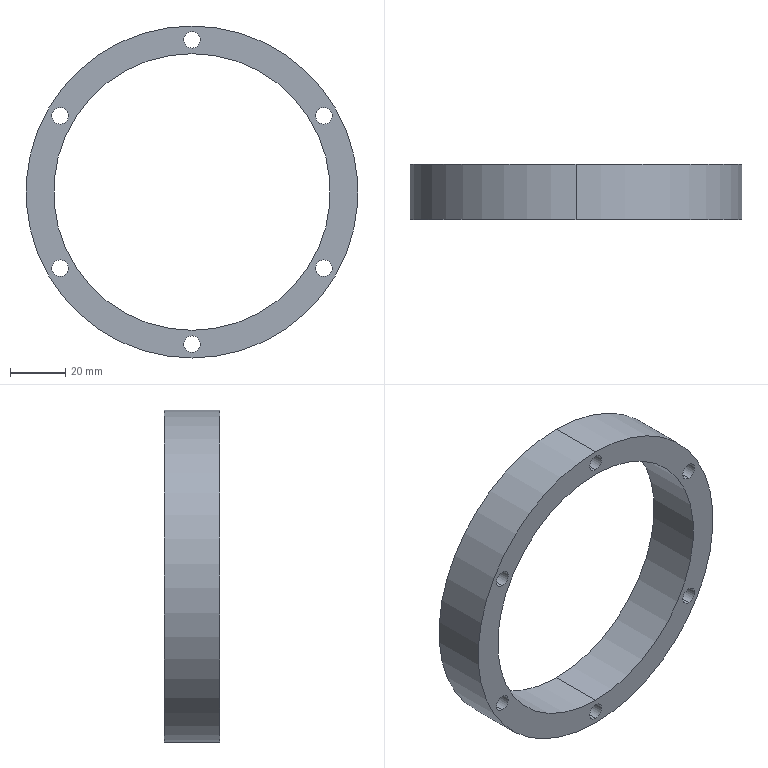Part | SolidWorks | features CirPattern 1, Extrusion 1, ICE 1 | 1 solid | 18 faces | box 120 x 20 x 120 mm | volume 65722 mm3 | cylinder 16 | plane 2 | commonest cylinder face diameters 6 x12 100 x2 120 x2
STEP:
#1=CARTESIAN_POINT('',(-47.631,0.,-30.5));
#2=VERTEX_POINT('',#1);
#3=CARTESIAN_POINT('',(-47.631,0.,-24.5));
#4=VERTEX_POINT('',#3);
#5=CARTESIAN_POINT('',(-47.631,0.,-27.5));
#6=DIRECTION('',(0.,1.,0.));
#7=DIRECTION('',(0.866,0.,0.5));
#8=AXIS2_PLACEMENT_3D('',#5,#6,#7);
#9=CIRCLE('',#8,3.);
#10=EDGE_CURVE('',#2,#4,#9,.T.);
#11=ORIENTED_EDGE('',*,*,#10,.F.);
#12=CARTESIAN_POINT('',(-47.631,20.,-30.5));
#13=VERTEX_POINT('',#12);
#14=CARTESIAN_POINT('',(-47.631,0.,-30.5));
#15=DIRECTION('',(0.,1.,0.));
#16=VECTOR('',#15,1000.);
#17=LINE('',#14,#16);
#18=EDGE_CURVE('',#2,#13,#17,.T.);
#19=ORIENTED_EDGE('',*,*,#18,.T.);
#20=CARTESIAN_POINT('',(-47.631,20.,-24.5));
#21=VERTEX_POINT('',#20);
#22=CARTESIAN_POINT('',(-47.631,20.,-27.5));
#23=DIRECTION('',(0.,1.,0.));
#24=DIRECTION('',(0.866,0.,0.5));
#25=AXIS2_PLACEMENT_3D('',#22,#23,#24);
#26=CIRCLE('',#25,3.);
#27=EDGE_CURVE('',#13,#21,#26,.T.);
#28=ORIENTED_EDGE('',*,*,#27,.T.);
#29=CARTESIAN_POINT('',(-47.631,0.,-24.5));
#30=DIRECTION('',(0.,1.,0.));
#31=VECTOR('',#30,1000.);
#32=LINE('',#29,#31);
#33=EDGE_CURVE('',#4,#21,#32,.T.);
#34=ORIENTED_EDGE('',*,*,#33,.F.);
#35=EDGE_LOOP('',(#11,#19,#28,#34));
#36=FACE_OUTER_BOUND('',#35,.T.);
#37=CARTESIAN_POINT('',(-47.631,0.,-27.5));
#38=DIRECTION('',(0.,1.,0.));
#39=DIRECTION('',(0.,0.,1.));
#40=AXIS2_PLACEMENT_3D('',#37,#38,#39);
#41=CYLINDRICAL_SURFACE('',#40,3.);
#42=ADVANCED_FACE('',(#36),#41,.F.);
#43=CARTESIAN_POINT('',(-47.631,0.,24.5));
#44=VERTEX_POINT('',#43);
#45=CARTESIAN_POINT('',(-47.631,0.,30.5));
#46=VERTEX_POINT('',#45);
#47=CARTESIAN_POINT('',(-47.631,0.,27.5));
#48=DIRECTION('',(0.,1.,0.));
#49=DIRECTION('',(0.866,0.,-0.5));
#50=AXIS2_PLACEMENT_3D('',#47,#48,#49);
#51=CIRCLE('',#50,3.);
#52=EDGE_CURVE('',#44,#46,#51,.T.);
#53=ORIENTED_EDGE('',*,*,#52,.F.);
#54=CARTESIAN_POINT('',(-47.631,20.,24.5));
#55=VERTEX_POINT('',#54);
#56=CARTESIAN_POINT('',(-47.631,0.,24.5));
#57=DIRECTION('',(0.,1.,0.));
#58=VECTOR('',#57,1000.);
#59=LINE('',#56,#58);
#60=EDGE_CURVE('',#44,#55,#59,.T.);
#61=ORIENTED_EDGE('',*,*,#60,.T.);
#62=CARTESIAN_POINT('',(-47.631,20.,30.5));
#63=VERTEX_POINT('',#62);
#64=CARTESIAN_POINT('',(-47.631,20.,27.5));
#65=DIRECTION('',(0.,1.,0.));
#66=DIRECTION('',(0.866,0.,-0.5));
#67=AXIS2_PLACEMENT_3D('',#64,#65,#66);
#68=CIRCLE('',#67,3.);
#69=EDGE_CURVE('',#55,#63,#68,.T.);
#70=ORIENTED_EDGE('',*,*,#69,.T.);
#71=CARTESIAN_POINT('',(-47.631,0.,30.5));
#72=DIRECTION('',(0.,1.,0.));
#73=VECTOR('',#72,1000.);
#74=LINE('',#71,#73);
#75=EDGE_CURVE('',#46,#63,#74,.T.);
#76=ORIENTED_EDGE('',*,*,#75,.F.);
#77=EDGE_LOOP('',(#53,#61,#70,#76));
#78=FACE_OUTER_BOUND('',#77,.T.);
#79=CARTESIAN_POINT('',(-47.631,0.,27.5));
#80=DIRECTION('',(0.,1.,0.));
#81=DIRECTION('',(0.,0.,1.));
#82=AXIS2_PLACEMENT_3D('',#79,#80,#81);
#83=CYLINDRICAL_SURFACE('',#82,3.);
#84=ADVANCED_FACE('',(#78),#83,.F.);
#85=CARTESIAN_POINT('',(0.,0.,52.));
#86=VERTEX_POINT('',#85);
#87=CARTESIAN_POINT('',(0.,0.,58.));
#88=VERTEX_POINT('',#87);
#89=CARTESIAN_POINT('',(0.,0.,55.));
#90=DIRECTION('',(0.,1.,0.));
#91=DIRECTION('',(0.,0.,-1.));
#92=AXIS2_PLACEMENT_3D('',#89,#90,#91);
#93=CIRCLE('',#92,3.);
#94=EDGE_CURVE('',#86,#88,#93,.T.);
#95=ORIENTED_EDGE('',*,*,#94,.F.);
#96=CARTESIAN_POINT('',(0.,20.,52.));
#97=VERTEX_POINT('',#96);
#98=CARTESIAN_POINT('',(0.,0.,52.));
#99=DIRECTION('',(0.,1.,0.));
#100=VECTOR('',#99,1000.);
#101=LINE('',#98,#100);
#102=EDGE_CURVE('',#86,#97,#101,.T.);
#103=ORIENTED_EDGE('',*,*,#102,.T.);
#104=CARTESIAN_POINT('',(0.,20.,58.));
#105=VERTEX_POINT('',#104);
#106=CARTESIAN_POINT('',(0.,20.,55.));
#107=DIRECTION('',(0.,1.,0.));
#108=DIRECTION('',(0.,0.,-1.));
#109=AXIS2_PLACEMENT_3D('',#106,#107,#108);
#110=CIRCLE('',#109,3.);
#111=EDGE_CURVE('',#97,#105,#110,.T.);
#112=ORIENTED_EDGE('',*,*,#111,.T.);
#113=CARTESIAN_POINT('',(0.,0.,58.));
#114=DIRECTION('',(0.,1.,0.));
#115=VECTOR('',#114,1000.);
#116=LINE('',#113,#115);
#117=EDGE_CURVE('',#88,#105,#116,.T.);
#118=ORIENTED_EDGE('',*,*,#117,.F.);
#119=EDGE_LOOP('',(#95,#103,#112,#118));
#120=FACE_OUTER_BOUND('',#119,.T.);
#121=CARTESIAN_POINT('',(0.,0.,55.));
#122=DIRECTION('',(0.,1.,0.));
#123=DIRECTION('',(0.,0.,1.));
#124=AXIS2_PLACEMENT_3D('',#121,#122,#123);
#125=CYLINDRICAL_SURFACE('',#124,3.);
#126=ADVANCED_FACE('',(#120),#125,.F.);
#127=CARTESIAN_POINT('',(47.631,0.,24.5));
#128=VERTEX_POINT('',#127);
#129=CARTESIAN_POINT('',(47.631,0.,30.5));
#130=VERTEX_POINT('',#129);
#131=CARTESIAN_POINT('',(47.631,0.,27.5));
#132=DIRECTION('',(0.,1.,0.));
#133=DIRECTION('',(-0.866,0.,-0.5));
#134=AXIS2_PLACEMENT_3D('',#131,#132,#133);
#135=CIRCLE('',#134,3.);
#136=EDGE_CURVE('',#128,#130,#135,.T.);
#137=ORIENTED_EDGE('',*,*,#136,.F.);
#138=CARTESIAN_POINT('',(47.631,20.,24.5));
#139=VERTEX_POINT('',#138);
#140=CARTESIAN_POINT('',(47.631,0.,24.5));
#141=DIRECTION('',(0.,1.,0.));
#142=VECTOR('',#141,1000.);
#143=LINE('',#140,#142);
#144=EDGE_CURVE('',#128,#139,#143,.T.);
#145=ORIENTED_EDGE('',*,*,#144,.T.);
#146=CARTESIAN_POINT('',(47.631,20.,30.5));
#147=VERTEX_POINT('',#146);
#148=CARTESIAN_POINT('',(47.631,20.,27.5));
#149=DIRECTION('',(0.,1.,0.));
#150=DIRECTION('',(-0.866,0.,-0.5));
#151=AXIS2_PLACEMENT_3D('',#148,#149,#150);
#152=CIRCLE('',#151,3.);
#153=EDGE_CURVE('',#139,#147,#152,.T.);
#154=ORIENTED_EDGE('',*,*,#153,.T.);
#155=CARTESIAN_POINT('',(47.631,0.,30.5));
#156=DIRECTION('',(0.,1.,0.));
#157=VECTOR('',#156,1000.);
#158=LINE('',#155,#157);
#159=EDGE_CURVE('',#130,#147,#158,.T.);
#160=ORIENTED_EDGE('',*,*,#159,.F.);
#161=EDGE_LOOP('',(#137,#145,#154,#160));
#162=FACE_OUTER_BOUND('',#161,.T.);
#163=CARTESIAN_POINT('',(47.631,0.,27.5));
#164=DIRECTION('',(0.,1.,0.));
#165=DIRECTION('',(0.,0.,1.));
#166=AXIS2_PLACEMENT_3D('',#163,#164,#165);
#167=CYLINDRICAL_SURFACE('',#166,3.);
#168=ADVANCED_FACE('',(#162),#167,.F.);
#169=CARTESIAN_POINT('',(47.631,0.,-30.5));
#170=VERTEX_POINT('',#169);
#171=CARTESIAN_POINT('',(47.631,0.,-24.5));
#172=VERTEX_POINT('',#171);
#173=CARTESIAN_POINT('',(47.631,0.,-27.5));
#174=DIRECTION('',(0.,1.,0.));
#175=DIRECTION('',(-0.866,0.,0.5));
#176=AXIS2_PLACEMENT_3D('',#173,#174,#175);
#177=CIRCLE('',#176,3.);
#178=EDGE_CURVE('',#170,#172,#177,.T.);
#179=ORIENTED_EDGE('',*,*,#178,.F.);
#180=CARTESIAN_POINT('',(47.631,20.,-30.5));
#181=VERTEX_POINT('',#180);
#182=CARTESIAN_POINT('',(47.631,0.,-30.5));
#183=DIRECTION('',(0.,1.,0.));
#184=VECTOR('',#183,1000.);
#185=LINE('',#182,#184);
#186=EDGE_CURVE('',#170,#181,#185,.T.);
#187=ORIENTED_EDGE('',*,*,#186,.T.);
#188=CARTESIAN_POINT('',(47.631,20.,-24.5));
#189=VERTEX_POINT('',#188);
#190=CARTESIAN_POINT('',(47.631,20.,-27.5));
#191=DIRECTION('',(0.,1.,0.));
#192=DIRECTION('',(-0.866,0.,0.5));
#193=AXIS2_PLACEMENT_3D('',#190,#191,#192);
#194=CIRCLE('',#193,3.);
#195=EDGE_CURVE('',#181,#189,#194,.T.);
#196=ORIENTED_EDGE('',*,*,#195,.T.);
#197=CARTESIAN_POINT('',(47.631,0.,-24.5));
#198=DIRECTION('',(0.,1.,0.));
#199=VECTOR('',#198,1000.);
#200=LINE('',#197,#199);
#201=EDGE_CURVE('',#172,#189,#200,.T.);
#202=ORIENTED_EDGE('',*,*,#201,.F.);
#203=EDGE_LOOP('',(#179,#187,#196,#202));
#204=FACE_OUTER_BOUND('',#203,.T.);
#205=CARTESIAN_POINT('',(47.631,0.,-27.5));
#206=DIRECTION('',(0.,1.,0.));
#207=DIRECTION('',(0.,0.,1.));
#208=AXIS2_PLACEMENT_3D('',#205,#206,#207);
#209=CYLINDRICAL_SURFACE('',#208,3.);
#210=ADVANCED_FACE('',(#204),#209,.F.);
#211=CARTESIAN_POINT('',(0.,0.,-58.));
#212=VERTEX_POINT('',#211);
#213=CARTESIAN_POINT('',(0.,0.,-52.));
#214=VERTEX_POINT('',#213);
#215=CARTESIAN_POINT('',(0.,0.,-55.));
#216=DIRECTION('',(0.,1.,0.));
#217=DIRECTION('',(0.,0.,1.));
#218=AXIS2_PLACEMENT_3D('',#215,#216,#217);
#219=CIRCLE('',#218,3.);
#220=EDGE_CURVE('',#212,#214,#219,.T.);
#221=ORIENTED_EDGE('',*,*,#220,.F.);
#222=CARTESIAN_POINT('',(0.,20.,-58.));
#223=VERTEX_POINT('',#222);
#224=CARTESIAN_POINT('',(0.,0.,-58.));
#225=DIRECTION('',(0.,1.,0.));
#226=VECTOR('',#225,1000.);
#227=LINE('',#224,#226);
#228=EDGE_CURVE('',#212,#223,#227,.T.);
#229=ORIENTED_EDGE('',*,*,#228,.T.);
#230=CARTESIAN_POINT('',(0.,20.,-52.));
#231=VERTEX_POINT('',#230);
#232=CARTESIAN_POINT('',(0.,20.,-55.));
#233=DIRECTION('',(0.,1.,0.));
#234=DIRECTION('',(0.,0.,1.));
#235=AXIS2_PLACEMENT_3D('',#232,#233,#234);
#236=CIRCLE('',#235,3.);
#237=EDGE_CURVE('',#223,#231,#236,.T.);
#238=ORIENTED_EDGE('',*,*,#237,.T.);
#239=CARTESIAN_POINT('',(0.,0.,-52.));
#240=DIRECTION('',(0.,1.,0.));
#241=VECTOR('',#240,1000.);
#242=LINE('',#239,#241);
#243=EDGE_CURVE('',#214,#231,#242,.T.);
#244=ORIENTED_EDGE('',*,*,#243,.F.);
#245=EDGE_LOOP('',(#221,#229,#238,#244));
#246=FACE_OUTER_BOUND('',#245,.T.);
#247=CARTESIAN_POINT('',(0.,0.,-55.));
#248=DIRECTION('',(0.,1.,0.));
#249=DIRECTION('',(0.,0.,1.));
#250=AXIS2_PLACEMENT_3D('',#247,#248,#249);
#251=CYLINDRICAL_SURFACE('',#250,3.);
#252=ADVANCED_FACE('',(#246),#251,.F.);
#253=CARTESIAN_POINT('',(0.,20.,-50.));
#254=VERTEX_POINT('',#253);
#255=CARTESIAN_POINT('',(0.,20.,50.));
#256=VERTEX_POINT('',#255);
#257=CARTESIAN_POINT('',(0.,20.,0.));
#258=DIRECTION('',(0.,1.,0.));
#259=DIRECTION('',(0.,0.,1.));
#260=AXIS2_PLACEMENT_3D('',#257,#258,#259);
#261=CIRCLE('',#260,50.);
#262=EDGE_CURVE('',#254,#256,#261,.T.);
#263=ORIENTED_EDGE('',*,*,#262,.T.);
#264=CARTESIAN_POINT('',(0.,0.,50.));
#265=VERTEX_POINT('',#264);
#266=CARTESIAN_POINT('',(0.,20.,50.));
#267=DIRECTION('',(0.,-1.,0.));
#268=VECTOR('',#267,1000.);
#269=LINE('',#266,#268);
#270=EDGE_CURVE('',#256,#265,#269,.T.);
#271=ORIENTED_EDGE('',*,*,#270,.T.);
#272=CARTESIAN_POINT('',(0.,0.,-50.));
#273=VERTEX_POINT('',#272);
#274=CARTESIAN_POINT('',(0.,0.,0.));
#275=DIRECTION('',(0.,1.,0.));
#276=DIRECTION('',(0.,0.,1.));
#277=AXIS2_PLACEMENT_3D('',#274,#275,#276);
#278=CIRCLE('',#277,50.);
#279=EDGE_CURVE('',#273,#265,#278,.T.);
#280=ORIENTED_EDGE('',*,*,#279,.F.);
#281=CARTESIAN_POINT('',(0.,20.,-50.));
#282=DIRECTION('',(0.,-1.,0.));
#283=VECTOR('',#282,1000.);
#284=LINE('',#281,#283);
#285=EDGE_CURVE('',#254,#273,#284,.T.);
#286=ORIENTED_EDGE('',*,*,#285,.F.);
#287=EDGE_LOOP('',(#263,#271,#280,#286));
#288=FACE_OUTER_BOUND('',#287,.T.);
#289=CARTESIAN_POINT('',(0.,20.,0.));
#290=DIRECTION('',(0.,-1.,0.));
#291=DIRECTION('',(0.,0.,-1.));
#292=AXIS2_PLACEMENT_3D('',#289,#290,#291);
#293=CYLINDRICAL_SURFACE('',#292,50.);
#294=ADVANCED_FACE('',(#288),#293,.F.);
#295=CARTESIAN_POINT('',(0.,20.,60.));
#296=VERTEX_POINT('',#295);
#297=CARTESIAN_POINT('',(0.,20.,-60.));
#298=VERTEX_POINT('',#297);
#299=CARTESIAN_POINT('',(0.,20.,0.));
#300=DIRECTION('',(0.,1.,0.));
#301=DIRECTION('',(0.,0.,1.));
#302=AXIS2_PLACEMENT_3D('',#299,#300,#301);
#303=CIRCLE('',#302,60.);
#304=EDGE_CURVE('',#296,#298,#303,.T.);
#305=ORIENTED_EDGE('',*,*,#304,.F.);
#306=CARTESIAN_POINT('',(0.,0.,60.));
#307=VERTEX_POINT('',#306);
#308=CARTESIAN_POINT('',(0.,20.,60.));
#309=DIRECTION('',(0.,-1.,0.));
#310=VECTOR('',#309,1000.);
#311=LINE('',#308,#310);
#312=EDGE_CURVE('',#296,#307,#311,.T.);
#313=ORIENTED_EDGE('',*,*,#312,.T.);
#314=CARTESIAN_POINT('',(0.,0.,-60.));
#315=VERTEX_POINT('',#314);
#316=CARTESIAN_POINT('',(0.,0.,0.));
#317=DIRECTION('',(0.,1.,0.));
#318=DIRECTION('',(0.,0.,1.));
#319=AXIS2_PLACEMENT_3D('',#316,#317,#318);
#320=CIRCLE('',#319,60.);
#321=EDGE_CURVE('',#307,#315,#320,.T.);
#322=ORIENTED_EDGE('',*,*,#321,.T.);
#323=CARTESIAN_POINT('',(0.,20.,-60.));
#324=DIRECTION('',(0.,-1.,0.));
#325=VECTOR('',#324,1000.);
#326=LINE('',#323,#325);
#327=EDGE_CURVE('',#298,#315,#326,.T.);
#328=ORIENTED_EDGE('',*,*,#327,.F.);
#329=EDGE_LOOP('',(#305,#313,#322,#328));
#330=FACE_OUTER_BOUND('',#329,.T.);
#331=CARTESIAN_POINT('',(0.,20.,0.));
#332=DIRECTION('',(0.,-1.,0.));
#333=DIRECTION('',(0.,0.,-1.));
#334=AXIS2_PLACEMENT_3D('',#331,#332,#333);
#335=CYLINDRICAL_SURFACE('',#334,60.);
#336=ADVANCED_FACE('',(#330),#335,.T.);
#337=CARTESIAN_POINT('',(-47.631,20.,-27.5));
#338=DIRECTION('',(0.,1.,0.));
#339=DIRECTION('',(0.866,0.,0.5));
#340=AXIS2_PLACEMENT_3D('',#337,#338,#339);
#341=CIRCLE('',#340,3.);
#342=EDGE_CURVE('',#21,#13,#341,.T.);
#343=ORIENTED_EDGE('',*,*,#342,.F.);
#344=ORIENTED_EDGE('',*,*,#27,.F.);
#345=EDGE_LOOP('',(#343,#344));
#346=FACE_BOUND('',#345,.T.);
#347=CARTESIAN_POINT('',(-47.631,20.,27.5));
#348=DIRECTION('',(0.,1.,0.));
#349=DIRECTION('',(0.866,0.,-0.5));
#350=AXIS2_PLACEMENT_3D('',#347,#348,#349);
#351=CIRCLE('',#350,3.);
#352=EDGE_CURVE('',#63,#55,#351,.T.);
#353=ORIENTED_EDGE('',*,*,#352,.F.);
#354=ORIENTED_EDGE('',*,*,#69,.F.);
#355=EDGE_LOOP('',(#353,#354));
#356=FACE_BOUND('',#355,.T.);
#357=CARTESIAN_POINT('',(0.,20.,55.));
#358=DIRECTION('',(0.,1.,0.));
#359=DIRECTION('',(0.,0.,-1.));
#360=AXIS2_PLACEMENT_3D('',#357,#358,#359);
#361=CIRCLE('',#360,3.);
#362=EDGE_CURVE('',#105,#97,#361,.T.);
#363=ORIENTED_EDGE('',*,*,#362,.F.);
#364=ORIENTED_EDGE('',*,*,#111,.F.);
#365=EDGE_LOOP('',(#363,#364));
#366=FACE_BOUND('',#365,.T.);
#367=CARTESIAN_POINT('',(47.631,20.,27.5));
#368=DIRECTION('',(0.,1.,0.));
#369=DIRECTION('',(-0.866,0.,-0.5));
#370=AXIS2_PLACEMENT_3D('',#367,#368,#369);
#371=CIRCLE('',#370,3.);
#372=EDGE_CURVE('',#147,#139,#371,.T.);
#373=ORIENTED_EDGE('',*,*,#372,.F.);
#374=ORIENTED_EDGE('',*,*,#153,.F.);
#375=EDGE_LOOP('',(#373,#374));
#376=FACE_BOUND('',#375,.T.);
#377=CARTESIAN_POINT('',(47.631,20.,-27.5));
#378=DIRECTION('',(0.,1.,0.));
#379=DIRECTION('',(-0.866,0.,0.5));
#380=AXIS2_PLACEMENT_3D('',#377,#378,#379);
#381=CIRCLE('',#380,3.);
#382=EDGE_CURVE('',#189,#181,#381,.T.);
#383=ORIENTED_EDGE('',*,*,#382,.F.);
#384=ORIENTED_EDGE('',*,*,#195,.F.);
#385=EDGE_LOOP('',(#383,#384));
#386=FACE_BOUND('',#385,.T.);
#387=CARTESIAN_POINT('',(0.,20.,-55.));
#388=DIRECTION('',(0.,1.,0.));
#389=DIRECTION('',(0.,0.,1.));
#390=AXIS2_PLACEMENT_3D('',#387,#388,#389);
#391=CIRCLE('',#390,3.);
#392=EDGE_CURVE('',#231,#223,#391,.T.);
#393=ORIENTED_EDGE('',*,*,#392,.F.);
#394=ORIENTED_EDGE('',*,*,#237,.F.);
#395=EDGE_LOOP('',(#393,#394));
#396=FACE_BOUND('',#395,.T.);
#397=CARTESIAN_POINT('',(0.,20.,0.));
#398=DIRECTION('',(0.,1.,0.));
#399=DIRECTION('',(0.,0.,1.));
#400=AXIS2_PLACEMENT_3D('',#397,#398,#399);
#401=CIRCLE('',#400,60.);
#402=EDGE_CURVE('',#298,#296,#401,.T.);
#403=ORIENTED_EDGE('',*,*,#402,.T.);
#404=ORIENTED_EDGE('',*,*,#304,.T.);
#405=EDGE_LOOP('',(#403,#404));
#406=FACE_OUTER_BOUND('',#405,.T.);
#407=ORIENTED_EDGE('',*,*,#262,.F.);
#408=CARTESIAN_POINT('',(0.,20.,0.));
#409=DIRECTION('',(0.,1.,0.));
#410=DIRECTION('',(0.,0.,1.));
#411=AXIS2_PLACEMENT_3D('',#408,#409,#410);
#412=CIRCLE('',#411,50.);
#413=EDGE_CURVE('',#256,#254,#412,.T.);
#414=ORIENTED_EDGE('',*,*,#413,.F.);
#415=EDGE_LOOP('',(#407,#414));
#416=FACE_BOUND('',#415,.T.);
#417=CARTESIAN_POINT('',(0.,20.,0.));
#418=DIRECTION('',(0.,1.,0.));
#419=DIRECTION('',(0.,0.,1.));
#420=AXIS2_PLACEMENT_3D('',#417,#418,#419);
#421=PLANE('',#420);
#422=ADVANCED_FACE('',(#346,#356,#366,#376,#386,#396,#406,#416),#421,.T.);
#423=CARTESIAN_POINT('',(-47.631,0.,-27.5));
#424=DIRECTION('',(0.,1.,0.));
#425=DIRECTION('',(0.866,0.,0.5));
#426=AXIS2_PLACEMENT_3D('',#423,#424,#425);
#427=CIRCLE('',#426,3.);
#428=EDGE_CURVE('',#4,#2,#427,.T.);
#429=ORIENTED_EDGE('',*,*,#428,.T.);
#430=ORIENTED_EDGE('',*,*,#10,.T.);
#431=EDGE_LOOP('',(#429,#430));
#432=FACE_BOUND('',#431,.T.);
#433=CARTESIAN_POINT('',(-47.631,0.,27.5));
#434=DIRECTION('',(0.,1.,0.));
#435=DIRECTION('',(0.866,0.,-0.5));
#436=AXIS2_PLACEMENT_3D('',#433,#434,#435);
#437=CIRCLE('',#436,3.);
#438=EDGE_CURVE('',#46,#44,#437,.T.);
#439=ORIENTED_EDGE('',*,*,#438,.T.);
#440=ORIENTED_EDGE('',*,*,#52,.T.);
#441=EDGE_LOOP('',(#439,#440));
#442=FACE_BOUND('',#441,.T.);
#443=CARTESIAN_POINT('',(0.,0.,55.));
#444=DIRECTION('',(0.,1.,0.));
#445=DIRECTION('',(0.,0.,-1.));
#446=AXIS2_PLACEMENT_3D('',#443,#444,#445);
#447=CIRCLE('',#446,3.);
#448=EDGE_CURVE('',#88,#86,#447,.T.);
#449=ORIENTED_EDGE('',*,*,#448,.T.);
#450=ORIENTED_EDGE('',*,*,#94,.T.);
#451=EDGE_LOOP('',(#449,#450));
#452=FACE_BOUND('',#451,.T.);
#453=CARTESIAN_POINT('',(47.631,0.,27.5));
#454=DIRECTION('',(0.,1.,0.));
#455=DIRECTION('',(-0.866,0.,-0.5));
#456=AXIS2_PLACEMENT_3D('',#453,#454,#455);
#457=CIRCLE('',#456,3.);
#458=EDGE_CURVE('',#130,#128,#457,.T.);
#459=ORIENTED_EDGE('',*,*,#458,.T.);
#460=ORIENTED_EDGE('',*,*,#136,.T.);
#461=EDGE_LOOP('',(#459,#460));
#462=FACE_BOUND('',#461,.T.);
#463=CARTESIAN_POINT('',(47.631,0.,-27.5));
#464=DIRECTION('',(0.,1.,0.));
#465=DIRECTION('',(-0.866,0.,0.5));
#466=AXIS2_PLACEMENT_3D('',#463,#464,#465);
#467=CIRCLE('',#466,3.);
#468=EDGE_CURVE('',#172,#170,#467,.T.);
#469=ORIENTED_EDGE('',*,*,#468,.T.);
#470=ORIENTED_EDGE('',*,*,#178,.T.);
#471=EDGE_LOOP('',(#469,#470));
#472=FACE_BOUND('',#471,.T.);
#473=CARTESIAN_POINT('',(0.,0.,-55.));
#474=DIRECTION('',(0.,1.,0.));
#475=DIRECTION('',(0.,0.,1.));
#476=AXIS2_PLACEMENT_3D('',#473,#474,#475);
#477=CIRCLE('',#476,3.);
#478=EDGE_CURVE('',#214,#212,#477,.T.);
#479=ORIENTED_EDGE('',*,*,#478,.T.);
#480=ORIENTED_EDGE('',*,*,#220,.T.);
#481=EDGE_LOOP('',(#479,#480));
#482=FACE_BOUND('',#481,.T.);
#483=CARTESIAN_POINT('',(0.,0.,0.));
#484=DIRECTION('',(0.,1.,0.));
#485=DIRECTION('',(0.,0.,1.));
#486=AXIS2_PLACEMENT_3D('',#483,#484,#485);
#487=CIRCLE('',#486,60.);
#488=EDGE_CURVE('',#315,#307,#487,.T.);
#489=ORIENTED_EDGE('',*,*,#488,.F.);
#490=ORIENTED_EDGE('',*,*,#321,.F.);
#491=EDGE_LOOP('',(#489,#490));
#492=FACE_OUTER_BOUND('',#491,.T.);
#493=ORIENTED_EDGE('',*,*,#279,.T.);
#494=CARTESIAN_POINT('',(0.,0.,0.));
#495=DIRECTION('',(0.,1.,0.));
#496=DIRECTION('',(0.,0.,1.));
#497=AXIS2_PLACEMENT_3D('',#494,#495,#496);
#498=CIRCLE('',#497,50.);
#499=EDGE_CURVE('',#265,#273,#498,.T.);
#500=ORIENTED_EDGE('',*,*,#499,.T.);
#501=EDGE_LOOP('',(#493,#500));
#502=FACE_BOUND('',#501,.T.);
#503=CARTESIAN_POINT('',(0.,0.,0.));
#504=DIRECTION('',(0.,1.,0.));
#505=DIRECTION('',(0.,0.,1.));
#506=AXIS2_PLACEMENT_3D('',#503,#504,#505);
#507=PLANE('',#506);
#508=ADVANCED_FACE('',(#432,#442,#452,#462,#472,#482,#492,#502),#507,.F.);
#509=ORIENTED_EDGE('',*,*,#312,.F.);
#510=ORIENTED_EDGE('',*,*,#402,.F.);
#511=ORIENTED_EDGE('',*,*,#327,.T.);
#512=ORIENTED_EDGE('',*,*,#488,.T.);
#513=EDGE_LOOP('',(#509,#510,#511,#512));
#514=FACE_OUTER_BOUND('',#513,.T.);
#515=CARTESIAN_POINT('',(0.,20.,0.));
#516=DIRECTION('',(0.,-1.,0.));
#517=DIRECTION('',(0.,0.,-1.));
#518=AXIS2_PLACEMENT_3D('',#515,#516,#517);
#519=CYLINDRICAL_SURFACE('',#518,60.);
#520=ADVANCED_FACE('',(#514),#519,.T.);
#521=ORIENTED_EDGE('',*,*,#270,.F.);
#522=ORIENTED_EDGE('',*,*,#413,.T.);
#523=ORIENTED_EDGE('',*,*,#285,.T.);
#524=ORIENTED_EDGE('',*,*,#499,.F.);
#525=EDGE_LOOP('',(#521,#522,#523,#524));
#526=FACE_OUTER_BOUND('',#525,.T.);
#527=CARTESIAN_POINT('',(0.,20.,0.));
#528=DIRECTION('',(0.,-1.,0.));
#529=DIRECTION('',(0.,0.,-1.));
#530=AXIS2_PLACEMENT_3D('',#527,#528,#529);
#531=CYLINDRICAL_SURFACE('',#530,50.);
#532=ADVANCED_FACE('',(#526),#531,.F.);
#533=ORIENTED_EDGE('',*,*,#228,.F.);
#534=ORIENTED_EDGE('',*,*,#478,.F.);
#535=ORIENTED_EDGE('',*,*,#243,.T.);
#536=ORIENTED_EDGE('',*,*,#392,.T.);
#537=EDGE_LOOP('',(#533,#534,#535,#536));
#538=FACE_OUTER_BOUND('',#537,.T.);
#539=CARTESIAN_POINT('',(0.,0.,-55.));
#540=DIRECTION('',(0.,1.,0.));
#541=DIRECTION('',(0.,0.,1.));
#542=AXIS2_PLACEMENT_3D('',#539,#540,#541);
#543=CYLINDRICAL_SURFACE('',#542,3.);
#544=ADVANCED_FACE('',(#538),#543,.F.);
#545=ORIENTED_EDGE('',*,*,#186,.F.);
#546=ORIENTED_EDGE('',*,*,#468,.F.);
#547=ORIENTED_EDGE('',*,*,#201,.T.);
#548=ORIENTED_EDGE('',*,*,#382,.T.);
#549=EDGE_LOOP('',(#545,#546,#547,#548));
#550=FACE_OUTER_BOUND('',#549,.T.);
#551=CARTESIAN_POINT('',(47.631,0.,-27.5));
#552=DIRECTION('',(0.,1.,0.));
#553=DIRECTION('',(0.,0.,1.));
#554=AXIS2_PLACEMENT_3D('',#551,#552,#553);
#555=CYLINDRICAL_SURFACE('',#554,3.);
#556=ADVANCED_FACE('',(#550),#555,.F.);
#557=ORIENTED_EDGE('',*,*,#144,.F.);
#558=ORIENTED_EDGE('',*,*,#458,.F.);
#559=ORIENTED_EDGE('',*,*,#159,.T.);
#560=ORIENTED_EDGE('',*,*,#372,.T.);
#561=EDGE_LOOP('',(#557,#558,#559,#560));
#562=FACE_OUTER_BOUND('',#561,.T.);
#563=CARTESIAN_POINT('',(47.631,0.,27.5));
#564=DIRECTION('',(0.,1.,0.));
#565=DIRECTION('',(0.,0.,1.));
#566=AXIS2_PLACEMENT_3D('',#563,#564,#565);
#567=CYLINDRICAL_SURFACE('',#566,3.);
#568=ADVANCED_FACE('',(#562),#567,.F.);
#569=ORIENTED_EDGE('',*,*,#102,.F.);
#570=ORIENTED_EDGE('',*,*,#448,.F.);
#571=ORIENTED_EDGE('',*,*,#117,.T.);
#572=ORIENTED_EDGE('',*,*,#362,.T.);
#573=EDGE_LOOP('',(#569,#570,#571,#572));
#574=FACE_OUTER_BOUND('',#573,.T.);
#575=CARTESIAN_POINT('',(0.,0.,55.));
#576=DIRECTION('',(0.,1.,0.));
#577=DIRECTION('',(0.,0.,1.));
#578=AXIS2_PLACEMENT_3D('',#575,#576,#577);
#579=CYLINDRICAL_SURFACE('',#578,3.);
#580=ADVANCED_FACE('',(#574),#579,.F.);
#581=ORIENTED_EDGE('',*,*,#60,.F.);
#582=ORIENTED_EDGE('',*,*,#438,.F.);
#583=ORIENTED_EDGE('',*,*,#75,.T.);
#584=ORIENTED_EDGE('',*,*,#352,.T.);
#585=EDGE_LOOP('',(#581,#582,#583,#584));
#586=FACE_OUTER_BOUND('',#585,.T.);
#587=CARTESIAN_POINT('',(-47.631,0.,27.5));
#588=DIRECTION('',(0.,1.,0.));
#589=DIRECTION('',(0.,0.,1.));
#590=AXIS2_PLACEMENT_3D('',#587,#588,#589);
#591=CYLINDRICAL_SURFACE('',#590,3.);
#592=ADVANCED_FACE('',(#586),#591,.F.);
#593=ORIENTED_EDGE('',*,*,#18,.F.);
#594=ORIENTED_EDGE('',*,*,#428,.F.);
#595=ORIENTED_EDGE('',*,*,#33,.T.);
#596=ORIENTED_EDGE('',*,*,#342,.T.);
#597=EDGE_LOOP('',(#593,#594,#595,#596));
#598=FACE_OUTER_BOUND('',#597,.T.);
#599=CARTESIAN_POINT('',(-47.631,0.,-27.5));
#600=DIRECTION('',(0.,1.,0.));
#601=DIRECTION('',(0.,0.,1.));
#602=AXIS2_PLACEMENT_3D('',#599,#600,#601);
#603=CYLINDRICAL_SURFACE('',#602,3.);
#604=ADVANCED_FACE('',(#598),#603,.F.);
#605=CLOSED_SHELL('',(#42,#84,#126,#168,#210,#252,#294,#336,#422,#508,#520,#532,#544,#556,#568,#580,#592,#604));
#606=MANIFOLD_SOLID_BREP('',#605);
#607=CARTESIAN_POINT('',(0.,0.,0.));
#608=DIRECTION('',(0.,0.,1.));
#609=DIRECTION('',(1.,0.,0.));
#610=AXIS2_PLACEMENT_3D('',#607,#608,#609);
#611=(LENGTH_UNIT()NAMED_UNIT(*)SI_UNIT(.MILLI.,.METRE.));
#612=UNCERTAINTY_MEASURE_WITH_UNIT(LENGTH_MEASURE(0.00001),#611,'','');
#613=(NAMED_UNIT(*)PLANE_ANGLE_UNIT()SI_UNIT($,.RADIAN.));
#614=(NAMED_UNIT(*)SI_UNIT($,.STERADIAN.)SOLID_ANGLE_UNIT());
#615=(GEOMETRIC_REPRESENTATION_CONTEXT(3)GLOBAL_UNCERTAINTY_ASSIGNED_CONTEXT((#612))GLOBAL_UNIT_ASSIGNED_CONTEXT((#611,#613,#614))REPRESENTATION_CONTEXT('',''));
#616=ADVANCED_BREP_SHAPE_REPRESENTATION('',(#606,#610),#615);